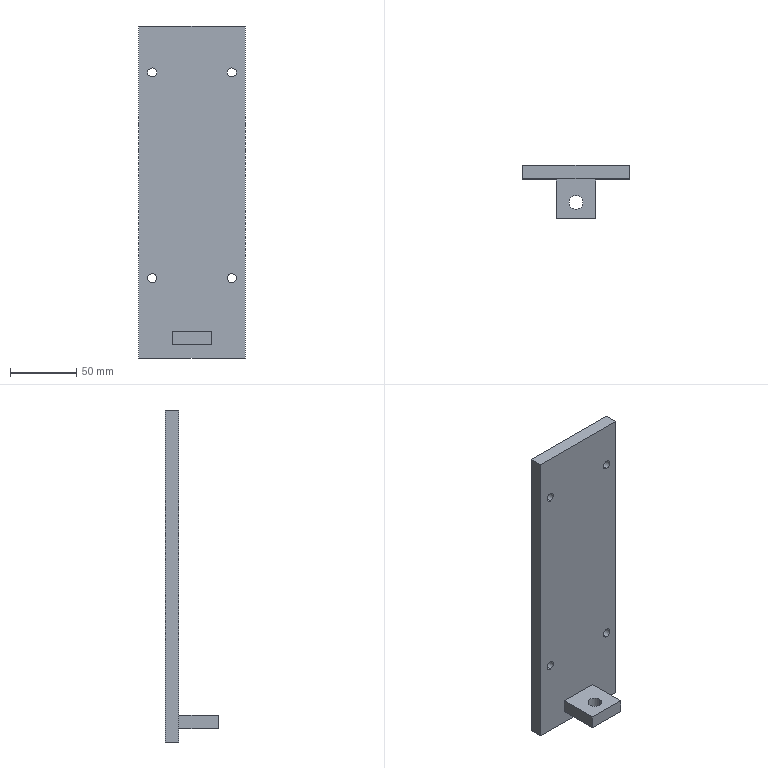Part | STEP file | X77-07008 | 1 solid | 21 faces | box 80 x 40 x 250 mm | volume 206681 mm3 | plane 11 | cylinder 10 | commonest cylinder face diameters 6.8 x8 10.5 x2
STEP:
#1=CARTESIAN_POINT('',(-328.942,-21.586,20.));
#2=VERTEX_POINT('',#1);
#3=CARTESIAN_POINT('',(-339.442,-21.586,20.));
#4=VERTEX_POINT('',#3);
#5=CARTESIAN_POINT('',(-334.192,-21.586,20.));
#6=DIRECTION('',(0.,0.,-1.));
#7=DIRECTION('',(-1.,0.,0.));
#8=AXIS2_PLACEMENT_3D('',#5,#6,#7);
#9=CIRCLE('',#8,5.25);
#10=EDGE_CURVE('',#2,#4,#9,.T.);
#11=ORIENTED_EDGE('',*,*,#10,.F.);
#12=CARTESIAN_POINT('',(-328.942,-21.586,10.));
#13=VERTEX_POINT('',#12);
#14=CARTESIAN_POINT('',(-328.942,-21.586,10.));
#15=DIRECTION('',(0.,0.,-1.));
#16=VECTOR('',#15,1000.);
#17=LINE('',#14,#16);
#18=EDGE_CURVE('',#2,#13,#17,.T.);
#19=ORIENTED_EDGE('',*,*,#18,.T.);
#20=CARTESIAN_POINT('',(-339.442,-21.586,10.));
#21=VERTEX_POINT('',#20);
#22=CARTESIAN_POINT('',(-334.192,-21.586,10.));
#23=DIRECTION('',(0.,0.,-1.));
#24=DIRECTION('',(-1.,0.,0.));
#25=AXIS2_PLACEMENT_3D('',#22,#23,#24);
#26=CIRCLE('',#25,5.25);
#27=EDGE_CURVE('',#13,#21,#26,.T.);
#28=ORIENTED_EDGE('',*,*,#27,.T.);
#29=CARTESIAN_POINT('',(-339.442,-21.586,10.));
#30=DIRECTION('',(0.,0.,-1.));
#31=VECTOR('',#30,1000.);
#32=LINE('',#29,#31);
#33=EDGE_CURVE('',#4,#21,#32,.T.);
#34=ORIENTED_EDGE('',*,*,#33,.F.);
#35=EDGE_LOOP('',(#11,#19,#28,#34));
#36=FACE_OUTER_BOUND('',#35,.T.);
#37=CARTESIAN_POINT('',(-334.192,-21.586,10.));
#38=DIRECTION('',(0.,0.,-1.));
#39=DIRECTION('',(-1.,0.,0.));
#40=AXIS2_PLACEMENT_3D('',#37,#38,#39);
#41=CYLINDRICAL_SURFACE('',#40,5.25);
#42=ADVANCED_FACE('',(#36),#41,.F.);
#43=CARTESIAN_POINT('',(-304.189,6.109,63.4));
#44=VERTEX_POINT('',#43);
#45=CARTESIAN_POINT('',(-304.189,6.109,56.6));
#46=VERTEX_POINT('',#45);
#47=CARTESIAN_POINT('',(-304.189,6.109,60.));
#48=DIRECTION('',(0.,-1.,0.));
#49=DIRECTION('',(1.,0.,0.));
#50=AXIS2_PLACEMENT_3D('',#47,#48,#49);
#51=CIRCLE('',#50,3.4);
#52=EDGE_CURVE('',#44,#46,#51,.T.);
#53=ORIENTED_EDGE('',*,*,#52,.F.);
#54=CARTESIAN_POINT('',(-304.189,-3.891,63.4));
#55=VERTEX_POINT('',#54);
#56=CARTESIAN_POINT('',(-304.189,-3.891,63.4));
#57=DIRECTION('',(0.,-1.,0.));
#58=VECTOR('',#57,1000.);
#59=LINE('',#56,#58);
#60=EDGE_CURVE('',#44,#55,#59,.T.);
#61=ORIENTED_EDGE('',*,*,#60,.T.);
#62=CARTESIAN_POINT('',(-304.189,-3.891,56.6));
#63=VERTEX_POINT('',#62);
#64=CARTESIAN_POINT('',(-304.189,-3.891,60.));
#65=DIRECTION('',(0.,-1.,0.));
#66=DIRECTION('',(0.,0.,-1.));
#67=AXIS2_PLACEMENT_3D('',#64,#65,#66);
#68=CIRCLE('',#67,3.4);
#69=EDGE_CURVE('',#55,#63,#68,.T.);
#70=ORIENTED_EDGE('',*,*,#69,.T.);
#71=CARTESIAN_POINT('',(-304.189,-3.891,56.6));
#72=DIRECTION('',(0.,-1.,0.));
#73=VECTOR('',#72,1000.);
#74=LINE('',#71,#73);
#75=EDGE_CURVE('',#46,#63,#74,.T.);
#76=ORIENTED_EDGE('',*,*,#75,.F.);
#77=EDGE_LOOP('',(#53,#61,#70,#76));
#78=FACE_OUTER_BOUND('',#77,.T.);
#79=CARTESIAN_POINT('',(-304.189,-3.891,60.));
#80=DIRECTION('',(0.,-1.,0.));
#81=DIRECTION('',(0.,0.,-1.));
#82=AXIS2_PLACEMENT_3D('',#79,#80,#81);
#83=CYLINDRICAL_SURFACE('',#82,3.4);
#84=ADVANCED_FACE('',(#78),#83,.F.);
#85=CARTESIAN_POINT('',(-364.189,6.109,63.4));
#86=VERTEX_POINT('',#85);
#87=CARTESIAN_POINT('',(-364.189,6.109,56.6));
#88=VERTEX_POINT('',#87);
#89=CARTESIAN_POINT('',(-364.189,6.109,60.));
#90=DIRECTION('',(0.,-1.,0.));
#91=DIRECTION('',(1.,0.,0.));
#92=AXIS2_PLACEMENT_3D('',#89,#90,#91);
#93=CIRCLE('',#92,3.4);
#94=EDGE_CURVE('',#86,#88,#93,.T.);
#95=ORIENTED_EDGE('',*,*,#94,.F.);
#96=CARTESIAN_POINT('',(-364.189,-3.891,63.4));
#97=VERTEX_POINT('',#96);
#98=CARTESIAN_POINT('',(-364.189,-3.891,63.4));
#99=DIRECTION('',(0.,-1.,0.));
#100=VECTOR('',#99,1000.);
#101=LINE('',#98,#100);
#102=EDGE_CURVE('',#86,#97,#101,.T.);
#103=ORIENTED_EDGE('',*,*,#102,.T.);
#104=CARTESIAN_POINT('',(-364.189,-3.891,56.6));
#105=VERTEX_POINT('',#104);
#106=CARTESIAN_POINT('',(-364.189,-3.891,60.));
#107=DIRECTION('',(0.,-1.,0.));
#108=DIRECTION('',(0.,0.,-1.));
#109=AXIS2_PLACEMENT_3D('',#106,#107,#108);
#110=CIRCLE('',#109,3.4);
#111=EDGE_CURVE('',#97,#105,#110,.T.);
#112=ORIENTED_EDGE('',*,*,#111,.T.);
#113=CARTESIAN_POINT('',(-364.189,-3.891,56.6));
#114=DIRECTION('',(0.,-1.,0.));
#115=VECTOR('',#114,1000.);
#116=LINE('',#113,#115);
#117=EDGE_CURVE('',#88,#105,#116,.T.);
#118=ORIENTED_EDGE('',*,*,#117,.F.);
#119=EDGE_LOOP('',(#95,#103,#112,#118));
#120=FACE_OUTER_BOUND('',#119,.T.);
#121=CARTESIAN_POINT('',(-364.189,-3.891,60.));
#122=DIRECTION('',(0.,-1.,0.));
#123=DIRECTION('',(0.,0.,-1.));
#124=AXIS2_PLACEMENT_3D('',#121,#122,#123);
#125=CYLINDRICAL_SURFACE('',#124,3.4);
#126=ADVANCED_FACE('',(#120),#125,.F.);
#127=CARTESIAN_POINT('',(-304.189,6.109,218.4));
#128=VERTEX_POINT('',#127);
#129=CARTESIAN_POINT('',(-304.189,6.109,211.6));
#130=VERTEX_POINT('',#129);
#131=CARTESIAN_POINT('',(-304.189,6.109,215.));
#132=DIRECTION('',(0.,-1.,0.));
#133=DIRECTION('',(1.,0.,0.));
#134=AXIS2_PLACEMENT_3D('',#131,#132,#133);
#135=CIRCLE('',#134,3.4);
#136=EDGE_CURVE('',#128,#130,#135,.T.);
#137=ORIENTED_EDGE('',*,*,#136,.F.);
#138=CARTESIAN_POINT('',(-304.189,-3.891,218.4));
#139=VERTEX_POINT('',#138);
#140=CARTESIAN_POINT('',(-304.189,-3.891,218.4));
#141=DIRECTION('',(0.,-1.,0.));
#142=VECTOR('',#141,1000.);
#143=LINE('',#140,#142);
#144=EDGE_CURVE('',#128,#139,#143,.T.);
#145=ORIENTED_EDGE('',*,*,#144,.T.);
#146=CARTESIAN_POINT('',(-304.189,-3.891,211.6));
#147=VERTEX_POINT('',#146);
#148=CARTESIAN_POINT('',(-304.189,-3.891,215.));
#149=DIRECTION('',(0.,-1.,0.));
#150=DIRECTION('',(0.,0.,-1.));
#151=AXIS2_PLACEMENT_3D('',#148,#149,#150);
#152=CIRCLE('',#151,3.4);
#153=EDGE_CURVE('',#139,#147,#152,.T.);
#154=ORIENTED_EDGE('',*,*,#153,.T.);
#155=CARTESIAN_POINT('',(-304.189,-3.891,211.6));
#156=DIRECTION('',(0.,-1.,0.));
#157=VECTOR('',#156,1000.);
#158=LINE('',#155,#157);
#159=EDGE_CURVE('',#130,#147,#158,.T.);
#160=ORIENTED_EDGE('',*,*,#159,.F.);
#161=EDGE_LOOP('',(#137,#145,#154,#160));
#162=FACE_OUTER_BOUND('',#161,.T.);
#163=CARTESIAN_POINT('',(-304.189,-3.891,215.));
#164=DIRECTION('',(0.,-1.,0.));
#165=DIRECTION('',(0.,0.,-1.));
#166=AXIS2_PLACEMENT_3D('',#163,#164,#165);
#167=CYLINDRICAL_SURFACE('',#166,3.4);
#168=ADVANCED_FACE('',(#162),#167,.F.);
#169=CARTESIAN_POINT('',(-364.189,6.109,218.4));
#170=VERTEX_POINT('',#169);
#171=CARTESIAN_POINT('',(-364.189,6.109,211.6));
#172=VERTEX_POINT('',#171);
#173=CARTESIAN_POINT('',(-364.189,6.109,215.));
#174=DIRECTION('',(0.,-1.,0.));
#175=DIRECTION('',(1.,0.,0.));
#176=AXIS2_PLACEMENT_3D('',#173,#174,#175);
#177=CIRCLE('',#176,3.4);
#178=EDGE_CURVE('',#170,#172,#177,.T.);
#179=ORIENTED_EDGE('',*,*,#178,.F.);
#180=CARTESIAN_POINT('',(-364.189,-3.891,218.4));
#181=VERTEX_POINT('',#180);
#182=CARTESIAN_POINT('',(-364.189,-3.891,218.4));
#183=DIRECTION('',(0.,-1.,0.));
#184=VECTOR('',#183,1000.);
#185=LINE('',#182,#184);
#186=EDGE_CURVE('',#170,#181,#185,.T.);
#187=ORIENTED_EDGE('',*,*,#186,.T.);
#188=CARTESIAN_POINT('',(-364.189,-3.891,211.6));
#189=VERTEX_POINT('',#188);
#190=CARTESIAN_POINT('',(-364.189,-3.891,215.));
#191=DIRECTION('',(0.,-1.,0.));
#192=DIRECTION('',(0.,0.,-1.));
#193=AXIS2_PLACEMENT_3D('',#190,#191,#192);
#194=CIRCLE('',#193,3.4);
#195=EDGE_CURVE('',#181,#189,#194,.T.);
#196=ORIENTED_EDGE('',*,*,#195,.T.);
#197=CARTESIAN_POINT('',(-364.189,-3.891,211.6));
#198=DIRECTION('',(0.,-1.,0.));
#199=VECTOR('',#198,1000.);
#200=LINE('',#197,#199);
#201=EDGE_CURVE('',#172,#189,#200,.T.);
#202=ORIENTED_EDGE('',*,*,#201,.F.);
#203=EDGE_LOOP('',(#179,#187,#196,#202));
#204=FACE_OUTER_BOUND('',#203,.T.);
#205=CARTESIAN_POINT('',(-364.189,-3.891,215.));
#206=DIRECTION('',(0.,-1.,0.));
#207=DIRECTION('',(0.,0.,-1.));
#208=AXIS2_PLACEMENT_3D('',#205,#206,#207);
#209=CYLINDRICAL_SURFACE('',#208,3.4);
#210=ADVANCED_FACE('',(#204),#209,.F.);
#211=CARTESIAN_POINT('',(-374.189,-3.891,0.));
#212=VERTEX_POINT('',#211);
#213=CARTESIAN_POINT('',(-294.189,-3.891,0.));
#214=VERTEX_POINT('',#213);
#215=CARTESIAN_POINT('',(-294.189,-3.891,0.));
#216=DIRECTION('',(1.,0.,0.));
#217=VECTOR('',#216,1000.);
#218=LINE('',#215,#217);
#219=EDGE_CURVE('',#212,#214,#218,.T.);
#220=ORIENTED_EDGE('',*,*,#219,.T.);
#221=CARTESIAN_POINT('',(-294.189,-3.891,250.));
#222=VERTEX_POINT('',#221);
#223=CARTESIAN_POINT('',(-294.189,-3.891,250.));
#224=DIRECTION('',(0.,0.,-1.));
#225=VECTOR('',#224,1000.);
#226=LINE('',#223,#225);
#227=EDGE_CURVE('',#222,#214,#226,.T.);
#228=ORIENTED_EDGE('',*,*,#227,.F.);
#229=CARTESIAN_POINT('',(-374.189,-3.891,250.));
#230=VERTEX_POINT('',#229);
#231=CARTESIAN_POINT('',(-294.189,-3.891,250.));
#232=DIRECTION('',(1.,0.,0.));
#233=VECTOR('',#232,1000.);
#234=LINE('',#231,#233);
#235=EDGE_CURVE('',#230,#222,#234,.T.);
#236=ORIENTED_EDGE('',*,*,#235,.F.);
#237=CARTESIAN_POINT('',(-374.189,-3.891,250.));
#238=DIRECTION('',(0.,0.,-1.));
#239=VECTOR('',#238,1000.);
#240=LINE('',#237,#239);
#241=EDGE_CURVE('',#230,#212,#240,.T.);
#242=ORIENTED_EDGE('',*,*,#241,.T.);
#243=EDGE_LOOP('',(#220,#228,#236,#242));
#244=FACE_OUTER_BOUND('',#243,.T.);
#245=CARTESIAN_POINT('',(-364.189,-3.891,215.));
#246=DIRECTION('',(0.,-1.,0.));
#247=DIRECTION('',(0.,0.,-1.));
#248=AXIS2_PLACEMENT_3D('',#245,#246,#247);
#249=CIRCLE('',#248,3.4);
#250=EDGE_CURVE('',#189,#181,#249,.T.);
#251=ORIENTED_EDGE('',*,*,#250,.F.);
#252=ORIENTED_EDGE('',*,*,#195,.F.);
#253=EDGE_LOOP('',(#251,#252));
#254=FACE_BOUND('',#253,.T.);
#255=CARTESIAN_POINT('',(-304.189,-3.891,215.));
#256=DIRECTION('',(0.,-1.,0.));
#257=DIRECTION('',(0.,0.,-1.));
#258=AXIS2_PLACEMENT_3D('',#255,#256,#257);
#259=CIRCLE('',#258,3.4);
#260=EDGE_CURVE('',#147,#139,#259,.T.);
#261=ORIENTED_EDGE('',*,*,#260,.F.);
#262=ORIENTED_EDGE('',*,*,#153,.F.);
#263=EDGE_LOOP('',(#261,#262));
#264=FACE_BOUND('',#263,.T.);
#265=CARTESIAN_POINT('',(-364.189,-3.891,60.));
#266=DIRECTION('',(0.,-1.,0.));
#267=DIRECTION('',(0.,0.,-1.));
#268=AXIS2_PLACEMENT_3D('',#265,#266,#267);
#269=CIRCLE('',#268,3.4);
#270=EDGE_CURVE('',#105,#97,#269,.T.);
#271=ORIENTED_EDGE('',*,*,#270,.F.);
#272=ORIENTED_EDGE('',*,*,#111,.F.);
#273=EDGE_LOOP('',(#271,#272));
#274=FACE_BOUND('',#273,.T.);
#275=CARTESIAN_POINT('',(-304.189,-3.891,60.));
#276=DIRECTION('',(0.,-1.,0.));
#277=DIRECTION('',(0.,0.,-1.));
#278=AXIS2_PLACEMENT_3D('',#275,#276,#277);
#279=CIRCLE('',#278,3.4);
#280=EDGE_CURVE('',#63,#55,#279,.T.);
#281=ORIENTED_EDGE('',*,*,#280,.F.);
#282=ORIENTED_EDGE('',*,*,#69,.F.);
#283=EDGE_LOOP('',(#281,#282));
#284=FACE_BOUND('',#283,.T.);
#285=CARTESIAN_POINT('',(-349.189,-3.891,20.));
#286=VERTEX_POINT('',#285);
#287=CARTESIAN_POINT('',(-349.189,-3.891,10.));
#288=VERTEX_POINT('',#287);
#289=CARTESIAN_POINT('',(-349.189,-3.891,20.));
#290=DIRECTION('',(0.,0.,-1.));
#291=VECTOR('',#290,1000.);
#292=LINE('',#289,#291);
#293=EDGE_CURVE('',#286,#288,#292,.T.);
#294=ORIENTED_EDGE('',*,*,#293,.F.);
#295=CARTESIAN_POINT('',(-319.189,-3.891,20.));
#296=VERTEX_POINT('',#295);
#297=CARTESIAN_POINT('',(-319.189,-3.891,20.));
#298=DIRECTION('',(-1.,0.,0.));
#299=VECTOR('',#298,1000.);
#300=LINE('',#297,#299);
#301=EDGE_CURVE('',#296,#286,#300,.T.);
#302=ORIENTED_EDGE('',*,*,#301,.F.);
#303=CARTESIAN_POINT('',(-319.189,-3.891,10.));
#304=VERTEX_POINT('',#303);
#305=CARTESIAN_POINT('',(-319.189,-3.891,20.));
#306=DIRECTION('',(0.,0.,1.));
#307=VECTOR('',#306,1000.);
#308=LINE('',#305,#307);
#309=EDGE_CURVE('',#304,#296,#308,.T.);
#310=ORIENTED_EDGE('',*,*,#309,.F.);
#311=CARTESIAN_POINT('',(-319.189,-3.891,10.));
#312=DIRECTION('',(1.,0.,0.));
#313=VECTOR('',#312,1000.);
#314=LINE('',#311,#313);
#315=EDGE_CURVE('',#288,#304,#314,.T.);
#316=ORIENTED_EDGE('',*,*,#315,.F.);
#317=EDGE_LOOP('',(#294,#302,#310,#316));
#318=FACE_BOUND('',#317,.T.);
#319=CARTESIAN_POINT('',(-294.189,-3.891,250.));
#320=DIRECTION('',(0.,1.,0.));
#321=DIRECTION('',(0.,0.,1.));
#322=AXIS2_PLACEMENT_3D('',#319,#320,#321);
#323=PLANE('',#322);
#324=ADVANCED_FACE('',(#244,#254,#264,#274,#284,#318),#323,.F.);
#325=CARTESIAN_POINT('',(-294.189,6.109,0.));
#326=VERTEX_POINT('',#325);
#327=CARTESIAN_POINT('',(-294.189,-3.891,0.));
#328=DIRECTION('',(0.,1.,0.));
#329=VECTOR('',#328,1000.);
#330=LINE('',#327,#329);
#331=EDGE_CURVE('',#214,#326,#330,.T.);
#332=ORIENTED_EDGE('',*,*,#331,.T.);
#333=CARTESIAN_POINT('',(-294.189,6.109,250.));
#334=VERTEX_POINT('',#333);
#335=CARTESIAN_POINT('',(-294.189,6.109,250.));
#336=DIRECTION('',(0.,0.,-1.));
#337=VECTOR('',#336,1000.);
#338=LINE('',#335,#337);
#339=EDGE_CURVE('',#334,#326,#338,.T.);
#340=ORIENTED_EDGE('',*,*,#339,.F.);
#341=CARTESIAN_POINT('',(-294.189,-3.891,250.));
#342=DIRECTION('',(0.,1.,0.));
#343=VECTOR('',#342,1000.);
#344=LINE('',#341,#343);
#345=EDGE_CURVE('',#222,#334,#344,.T.);
#346=ORIENTED_EDGE('',*,*,#345,.F.);
#347=ORIENTED_EDGE('',*,*,#227,.T.);
#348=EDGE_LOOP('',(#332,#340,#346,#347));
#349=FACE_OUTER_BOUND('',#348,.T.);
#350=CARTESIAN_POINT('',(-294.189,-3.891,250.));
#351=DIRECTION('',(-1.,0.,0.));
#352=DIRECTION('',(0.,0.,1.));
#353=AXIS2_PLACEMENT_3D('',#350,#351,#352);
#354=PLANE('',#353);
#355=ADVANCED_FACE('',(#349),#354,.F.);
#356=CARTESIAN_POINT('',(-304.189,6.109,60.));
#357=DIRECTION('',(0.,-1.,0.));
#358=DIRECTION('',(1.,0.,0.));
#359=AXIS2_PLACEMENT_3D('',#356,#357,#358);
#360=CIRCLE('',#359,3.4);
#361=EDGE_CURVE('',#46,#44,#360,.T.);
#362=ORIENTED_EDGE('',*,*,#361,.T.);
#363=ORIENTED_EDGE('',*,*,#52,.T.);
#364=EDGE_LOOP('',(#362,#363));
#365=FACE_BOUND('',#364,.T.);
#366=CARTESIAN_POINT('',(-364.189,6.109,60.));
#367=DIRECTION('',(0.,-1.,0.));
#368=DIRECTION('',(1.,0.,0.));
#369=AXIS2_PLACEMENT_3D('',#366,#367,#368);
#370=CIRCLE('',#369,3.4);
#371=EDGE_CURVE('',#88,#86,#370,.T.);
#372=ORIENTED_EDGE('',*,*,#371,.T.);
#373=ORIENTED_EDGE('',*,*,#94,.T.);
#374=EDGE_LOOP('',(#372,#373));
#375=FACE_BOUND('',#374,.T.);
#376=CARTESIAN_POINT('',(-304.189,6.109,215.));
#377=DIRECTION('',(0.,-1.,0.));
#378=DIRECTION('',(1.,0.,0.));
#379=AXIS2_PLACEMENT_3D('',#376,#377,#378);
#380=CIRCLE('',#379,3.4);
#381=EDGE_CURVE('',#130,#128,#380,.T.);
#382=ORIENTED_EDGE('',*,*,#381,.T.);
#383=ORIENTED_EDGE('',*,*,#136,.T.);
#384=EDGE_LOOP('',(#382,#383));
#385=FACE_BOUND('',#384,.T.);
#386=CARTESIAN_POINT('',(-364.189,6.109,215.));
#387=DIRECTION('',(0.,-1.,0.));
#388=DIRECTION('',(1.,0.,0.));
#389=AXIS2_PLACEMENT_3D('',#386,#387,#388);
#390=CIRCLE('',#389,3.4);
#391=EDGE_CURVE('',#172,#170,#390,.T.);
#392=ORIENTED_EDGE('',*,*,#391,.T.);
#393=ORIENTED_EDGE('',*,*,#178,.T.);
#394=EDGE_LOOP('',(#392,#393));
#395=FACE_BOUND('',#394,.T.);
#396=CARTESIAN_POINT('',(-374.189,6.109,0.));
#397=VERTEX_POINT('',#396);
#398=CARTESIAN_POINT('',(-294.189,6.109,0.));
#399=DIRECTION('',(-1.,0.,0.));
#400=VECTOR('',#399,1000.);
#401=LINE('',#398,#400);
#402=EDGE_CURVE('',#326,#397,#401,.T.);
#403=ORIENTED_EDGE('',*,*,#402,.T.);
#404=CARTESIAN_POINT('',(-374.189,6.109,250.));
#405=VERTEX_POINT('',#404);
#406=CARTESIAN_POINT('',(-374.189,6.109,250.));
#407=DIRECTION('',(0.,0.,-1.));
#408=VECTOR('',#407,1000.);
#409=LINE('',#406,#408);
#410=EDGE_CURVE('',#405,#397,#409,.T.);
#411=ORIENTED_EDGE('',*,*,#410,.F.);
#412=CARTESIAN_POINT('',(-294.189,6.109,250.));
#413=DIRECTION('',(-1.,0.,0.));
#414=VECTOR('',#413,1000.);
#415=LINE('',#412,#414);
#416=EDGE_CURVE('',#334,#405,#415,.T.);
#417=ORIENTED_EDGE('',*,*,#416,.F.);
#418=ORIENTED_EDGE('',*,*,#339,.T.);
#419=EDGE_LOOP('',(#403,#411,#417,#418));
#420=FACE_OUTER_BOUND('',#419,.T.);
#421=CARTESIAN_POINT('',(-294.189,6.109,250.));
#422=DIRECTION('',(0.,-1.,0.));
#423=DIRECTION('',(1.,0.,0.));
#424=AXIS2_PLACEMENT_3D('',#421,#422,#423);
#425=PLANE('',#424);
#426=ADVANCED_FACE('',(#365,#375,#385,#395,#420),#425,.F.);
#427=CARTESIAN_POINT('',(-374.189,-3.891,0.));
#428=DIRECTION('',(0.,-1.,0.));
#429=VECTOR('',#428,1000.);
#430=LINE('',#427,#429);
#431=EDGE_CURVE('',#397,#212,#430,.T.);
#432=ORIENTED_EDGE('',*,*,#431,.T.);
#433=ORIENTED_EDGE('',*,*,#241,.F.);
#434=CARTESIAN_POINT('',(-374.189,-3.891,250.));
#435=DIRECTION('',(0.,-1.,0.));
#436=VECTOR('',#435,1000.);
#437=LINE('',#434,#436);
#438=EDGE_CURVE('',#405,#230,#437,.T.);
#439=ORIENTED_EDGE('',*,*,#438,.F.);
#440=ORIENTED_EDGE('',*,*,#410,.T.);
#441=EDGE_LOOP('',(#432,#433,#439,#440));
#442=FACE_OUTER_BOUND('',#441,.T.);
#443=CARTESIAN_POINT('',(-374.189,-3.891,250.));
#444=DIRECTION('',(1.,0.,0.));
#445=DIRECTION('',(0.,0.,-1.));
#446=AXIS2_PLACEMENT_3D('',#443,#444,#445);
#447=PLANE('',#446);
#448=ADVANCED_FACE('',(#442),#447,.F.);
#449=ORIENTED_EDGE('',*,*,#345,.T.);
#450=ORIENTED_EDGE('',*,*,#416,.T.);
#451=ORIENTED_EDGE('',*,*,#438,.T.);
#452=ORIENTED_EDGE('',*,*,#235,.T.);
#453=EDGE_LOOP('',(#449,#450,#451,#452));
#454=FACE_OUTER_BOUND('',#453,.T.);
#455=CARTESIAN_POINT('',(-294.189,6.109,250.));
#456=DIRECTION('',(0.,0.,1.));
#457=DIRECTION('',(1.,0.,0.));
#458=AXIS2_PLACEMENT_3D('',#455,#456,#457);
#459=PLANE('',#458);
#460=ADVANCED_FACE('',(#454),#459,.T.);
#461=ORIENTED_EDGE('',*,*,#331,.F.);
#462=ORIENTED_EDGE('',*,*,#219,.F.);
#463=ORIENTED_EDGE('',*,*,#431,.F.);
#464=ORIENTED_EDGE('',*,*,#402,.F.);
#465=EDGE_LOOP('',(#461,#462,#463,#464));
#466=FACE_OUTER_BOUND('',#465,.T.);
#467=CARTESIAN_POINT('',(-294.189,6.109,0.));
#468=DIRECTION('',(0.,0.,1.));
#469=DIRECTION('',(1.,0.,0.));
#470=AXIS2_PLACEMENT_3D('',#467,#468,#469);
#471=PLANE('',#470);
#472=ADVANCED_FACE('',(#466),#471,.F.);
#473=ORIENTED_EDGE('',*,*,#186,.F.);
#474=ORIENTED_EDGE('',*,*,#391,.F.);
#475=ORIENTED_EDGE('',*,*,#201,.T.);
#476=ORIENTED_EDGE('',*,*,#250,.T.);
#477=EDGE_LOOP('',(#473,#474,#475,#476));
#478=FACE_OUTER_BOUND('',#477,.T.);
#479=CARTESIAN_POINT('',(-364.189,-3.891,215.));
#480=DIRECTION('',(0.,-1.,0.));
#481=DIRECTION('',(0.,0.,-1.));
#482=AXIS2_PLACEMENT_3D('',#479,#480,#481);
#483=CYLINDRICAL_SURFACE('',#482,3.4);
#484=ADVANCED_FACE('',(#478),#483,.F.);
#485=ORIENTED_EDGE('',*,*,#144,.F.);
#486=ORIENTED_EDGE('',*,*,#381,.F.);
#487=ORIENTED_EDGE('',*,*,#159,.T.);
#488=ORIENTED_EDGE('',*,*,#260,.T.);
#489=EDGE_LOOP('',(#485,#486,#487,#488));
#490=FACE_OUTER_BOUND('',#489,.T.);
#491=CARTESIAN_POINT('',(-304.189,-3.891,215.));
#492=DIRECTION('',(0.,-1.,0.));
#493=DIRECTION('',(0.,0.,-1.));
#494=AXIS2_PLACEMENT_3D('',#491,#492,#493);
#495=CYLINDRICAL_SURFACE('',#494,3.4);
#496=ADVANCED_FACE('',(#490),#495,.F.);
#497=ORIENTED_EDGE('',*,*,#102,.F.);
#498=ORIENTED_EDGE('',*,*,#371,.F.);
#499=ORIENTED_EDGE('',*,*,#117,.T.);
#500=ORIENTED_EDGE('',*,*,#270,.T.);
#501=EDGE_LOOP('',(#497,#498,#499,#500));
#502=FACE_OUTER_BOUND('',#501,.T.);
#503=CARTESIAN_POINT('',(-364.189,-3.891,60.));
#504=DIRECTION('',(0.,-1.,0.));
#505=DIRECTION('',(0.,0.,-1.));
#506=AXIS2_PLACEMENT_3D('',#503,#504,#505);
#507=CYLINDRICAL_SURFACE('',#506,3.4);
#508=ADVANCED_FACE('',(#502),#507,.F.);
#509=ORIENTED_EDGE('',*,*,#60,.F.);
#510=ORIENTED_EDGE('',*,*,#361,.F.);
#511=ORIENTED_EDGE('',*,*,#75,.T.);
#512=ORIENTED_EDGE('',*,*,#280,.T.);
#513=EDGE_LOOP('',(#509,#510,#511,#512));
#514=FACE_OUTER_BOUND('',#513,.T.);
#515=CARTESIAN_POINT('',(-304.189,-3.891,60.));
#516=DIRECTION('',(0.,-1.,0.));
#517=DIRECTION('',(0.,0.,-1.));
#518=AXIS2_PLACEMENT_3D('',#515,#516,#517);
#519=CYLINDRICAL_SURFACE('',#518,3.4);
#520=ADVANCED_FACE('',(#514),#519,.F.);
#521=ORIENTED_EDGE('',*,*,#293,.T.);
#522=CARTESIAN_POINT('',(-349.189,-33.891,10.));
#523=VERTEX_POINT('',#522);
#524=CARTESIAN_POINT('',(-349.189,-33.891,10.));
#525=DIRECTION('',(0.,1.,0.));
#526=VECTOR('',#525,1000.);
#527=LINE('',#524,#526);
#528=EDGE_CURVE('',#523,#288,#527,.T.);
#529=ORIENTED_EDGE('',*,*,#528,.F.);
#530=CARTESIAN_POINT('',(-349.189,-33.891,20.));
#531=VERTEX_POINT('',#530);
#532=CARTESIAN_POINT('',(-349.189,-33.891,20.));
#533=DIRECTION('',(0.,0.,-1.));
#534=VECTOR('',#533,1000.);
#535=LINE('',#532,#534);
#536=EDGE_CURVE('',#531,#523,#535,.T.);
#537=ORIENTED_EDGE('',*,*,#536,.F.);
#538=CARTESIAN_POINT('',(-349.189,-33.891,20.));
#539=DIRECTION('',(0.,1.,0.));
#540=VECTOR('',#539,1000.);
#541=LINE('',#538,#540);
#542=EDGE_CURVE('',#531,#286,#541,.T.);
#543=ORIENTED_EDGE('',*,*,#542,.T.);
#544=EDGE_LOOP('',(#521,#529,#537,#543));
#545=FACE_OUTER_BOUND('',#544,.T.);
#546=CARTESIAN_POINT('',(-349.189,-33.891,20.));
#547=DIRECTION('',(1.,0.,0.));
#548=DIRECTION('',(0.,0.,-1.));
#549=AXIS2_PLACEMENT_3D('',#546,#547,#548);
#550=PLANE('',#549);
#551=ADVANCED_FACE('',(#545),#550,.F.);
#552=CARTESIAN_POINT('',(-334.192,-21.586,10.));
#553=DIRECTION('',(0.,0.,-1.));
#554=DIRECTION('',(-1.,0.,0.));
#555=AXIS2_PLACEMENT_3D('',#552,#553,#554);
#556=CIRCLE('',#555,5.25);
#557=EDGE_CURVE('',#21,#13,#556,.T.);
#558=ORIENTED_EDGE('',*,*,#557,.F.);
#559=ORIENTED_EDGE('',*,*,#27,.F.);
#560=EDGE_LOOP('',(#558,#559));
#561=FACE_BOUND('',#560,.T.);
#562=ORIENTED_EDGE('',*,*,#315,.T.);
#563=CARTESIAN_POINT('',(-319.189,-33.891,10.));
#564=VERTEX_POINT('',#563);
#565=CARTESIAN_POINT('',(-319.189,-33.891,10.));
#566=DIRECTION('',(0.,1.,0.));
#567=VECTOR('',#566,1000.);
#568=LINE('',#565,#567);
#569=EDGE_CURVE('',#564,#304,#568,.T.);
#570=ORIENTED_EDGE('',*,*,#569,.F.);
#571=CARTESIAN_POINT('',(-319.189,-33.891,10.));
#572=DIRECTION('',(1.,0.,0.));
#573=VECTOR('',#572,1000.);
#574=LINE('',#571,#573);
#575=EDGE_CURVE('',#523,#564,#574,.T.);
#576=ORIENTED_EDGE('',*,*,#575,.F.);
#577=ORIENTED_EDGE('',*,*,#528,.T.);
#578=EDGE_LOOP('',(#562,#570,#576,#577));
#579=FACE_OUTER_BOUND('',#578,.T.);
#580=CARTESIAN_POINT('',(-319.189,-33.891,10.));
#581=DIRECTION('',(0.,0.,1.));
#582=DIRECTION('',(1.,0.,0.));
#583=AXIS2_PLACEMENT_3D('',#580,#581,#582);
#584=PLANE('',#583);
#585=ADVANCED_FACE('',(#561,#579),#584,.F.);
#586=ORIENTED_EDGE('',*,*,#309,.T.);
#587=CARTESIAN_POINT('',(-319.189,-33.891,20.));
#588=VERTEX_POINT('',#587);
#589=CARTESIAN_POINT('',(-319.189,-33.891,20.));
#590=DIRECTION('',(0.,1.,0.));
#591=VECTOR('',#590,1000.);
#592=LINE('',#589,#591);
#593=EDGE_CURVE('',#588,#296,#592,.T.);
#594=ORIENTED_EDGE('',*,*,#593,.F.);
#595=CARTESIAN_POINT('',(-319.189,-33.891,20.));
#596=DIRECTION('',(0.,0.,1.));
#597=VECTOR('',#596,1000.);
#598=LINE('',#595,#597);
#599=EDGE_CURVE('',#564,#588,#598,.T.);
#600=ORIENTED_EDGE('',*,*,#599,.F.);
#601=ORIENTED_EDGE('',*,*,#569,.T.);
#602=EDGE_LOOP('',(#586,#594,#600,#601));
#603=FACE_OUTER_BOUND('',#602,.T.);
#604=CARTESIAN_POINT('',(-319.189,-33.891,20.));
#605=DIRECTION('',(-1.,0.,0.));
#606=DIRECTION('',(0.,0.,1.));
#607=AXIS2_PLACEMENT_3D('',#604,#605,#606);
#608=PLANE('',#607);
#609=ADVANCED_FACE('',(#603),#608,.F.);
#610=CARTESIAN_POINT('',(-334.192,-21.586,20.));
#611=DIRECTION('',(0.,0.,-1.));
#612=DIRECTION('',(-1.,0.,0.));
#613=AXIS2_PLACEMENT_3D('',#610,#611,#612);
#614=CIRCLE('',#613,5.25);
#615=EDGE_CURVE('',#4,#2,#614,.T.);
#616=ORIENTED_EDGE('',*,*,#615,.T.);
#617=ORIENTED_EDGE('',*,*,#10,.T.);
#618=EDGE_LOOP('',(#616,#617));
#619=FACE_BOUND('',#618,.T.);
#620=ORIENTED_EDGE('',*,*,#301,.T.);
#621=ORIENTED_EDGE('',*,*,#542,.F.);
#622=CARTESIAN_POINT('',(-319.189,-33.891,20.));
#623=DIRECTION('',(-1.,0.,0.));
#624=VECTOR('',#623,1000.);
#625=LINE('',#622,#624);
#626=EDGE_CURVE('',#588,#531,#625,.T.);
#627=ORIENTED_EDGE('',*,*,#626,.F.);
#628=ORIENTED_EDGE('',*,*,#593,.T.);
#629=EDGE_LOOP('',(#620,#621,#627,#628));
#630=FACE_OUTER_BOUND('',#629,.T.);
#631=CARTESIAN_POINT('',(-319.189,-33.891,20.));
#632=DIRECTION('',(0.,0.,-1.));
#633=DIRECTION('',(-1.,0.,0.));
#634=AXIS2_PLACEMENT_3D('',#631,#632,#633);
#635=PLANE('',#634);
#636=ADVANCED_FACE('',(#619,#630),#635,.F.);
#637=ORIENTED_EDGE('',*,*,#536,.T.);
#638=ORIENTED_EDGE('',*,*,#575,.T.);
#639=ORIENTED_EDGE('',*,*,#599,.T.);
#640=ORIENTED_EDGE('',*,*,#626,.T.);
#641=EDGE_LOOP('',(#637,#638,#639,#640));
#642=FACE_OUTER_BOUND('',#641,.T.);
#643=CARTESIAN_POINT('',(-349.189,-33.891,10.));
#644=DIRECTION('',(0.,1.,0.));
#645=DIRECTION('',(0.,0.,1.));
#646=AXIS2_PLACEMENT_3D('',#643,#644,#645);
#647=PLANE('',#646);
#648=ADVANCED_FACE('',(#642),#647,.F.);
#649=ORIENTED_EDGE('',*,*,#18,.F.);
#650=ORIENTED_EDGE('',*,*,#615,.F.);
#651=ORIENTED_EDGE('',*,*,#33,.T.);
#652=ORIENTED_EDGE('',*,*,#557,.T.);
#653=EDGE_LOOP('',(#649,#650,#651,#652));
#654=FACE_OUTER_BOUND('',#653,.T.);
#655=CARTESIAN_POINT('',(-334.192,-21.586,10.));
#656=DIRECTION('',(0.,0.,-1.));
#657=DIRECTION('',(-1.,0.,0.));
#658=AXIS2_PLACEMENT_3D('',#655,#656,#657);
#659=CYLINDRICAL_SURFACE('',#658,5.25);
#660=ADVANCED_FACE('',(#654),#659,.F.);
#661=CLOSED_SHELL('',(#42,#84,#126,#168,#210,#324,#355,#426,#448,#460,#472,#484,#496,#508,#520,#551,#585,#609,#636,#648,#660));
#662=MANIFOLD_SOLID_BREP('',#661);
#663=CARTESIAN_POINT('',(0.,0.,0.));
#664=DIRECTION('',(0.,0.,1.));
#665=DIRECTION('',(1.,0.,0.));
#666=AXIS2_PLACEMENT_3D('',#663,#664,#665);
#667=(LENGTH_UNIT()NAMED_UNIT(*)SI_UNIT(.MILLI.,.METRE.));
#668=UNCERTAINTY_MEASURE_WITH_UNIT(LENGTH_MEASURE(0.00001),#667,'','');
#669=(NAMED_UNIT(*)PLANE_ANGLE_UNIT()SI_UNIT($,.RADIAN.));
#670=(NAMED_UNIT(*)SI_UNIT($,.STERADIAN.)SOLID_ANGLE_UNIT());
#671=(GEOMETRIC_REPRESENTATION_CONTEXT(3)GLOBAL_UNCERTAINTY_ASSIGNED_CONTEXT((#668))GLOBAL_UNIT_ASSIGNED_CONTEXT((#667,#669,#670))REPRESENTATION_CONTEXT('',''));
#672=ADVANCED_BREP_SHAPE_REPRESENTATION('',(#662,#666),#671);